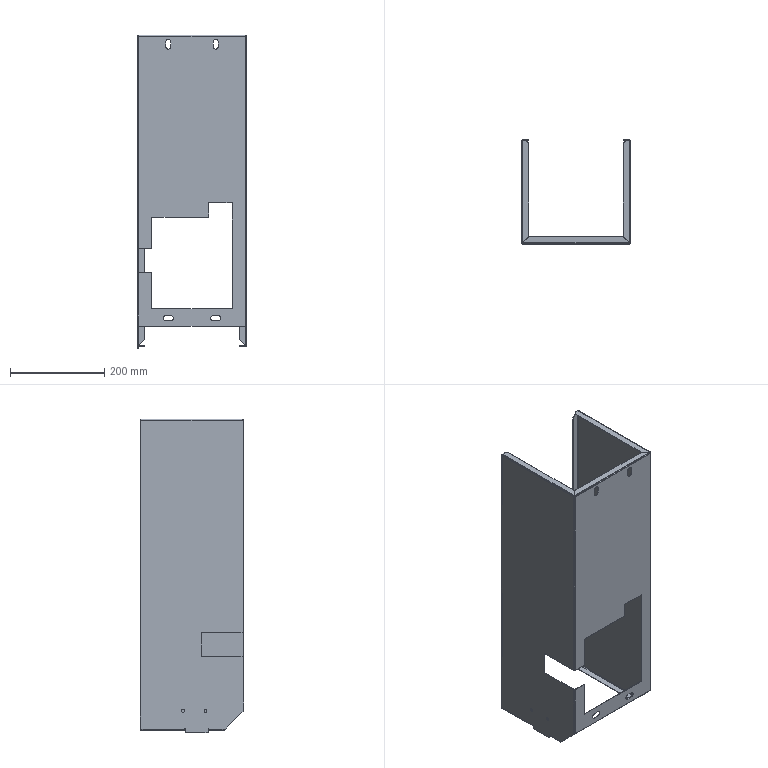Part | SolidWorks | features BaseBody 1 | 1 solid | 174 faces | box 230 x 220 x 664 mm | volume 415527 mm3 | plane 118 | cylinder 44 | spline 12 | commonest cylinder face diameters 2 x13 4 x13 11 x10 6 x4 16 x4